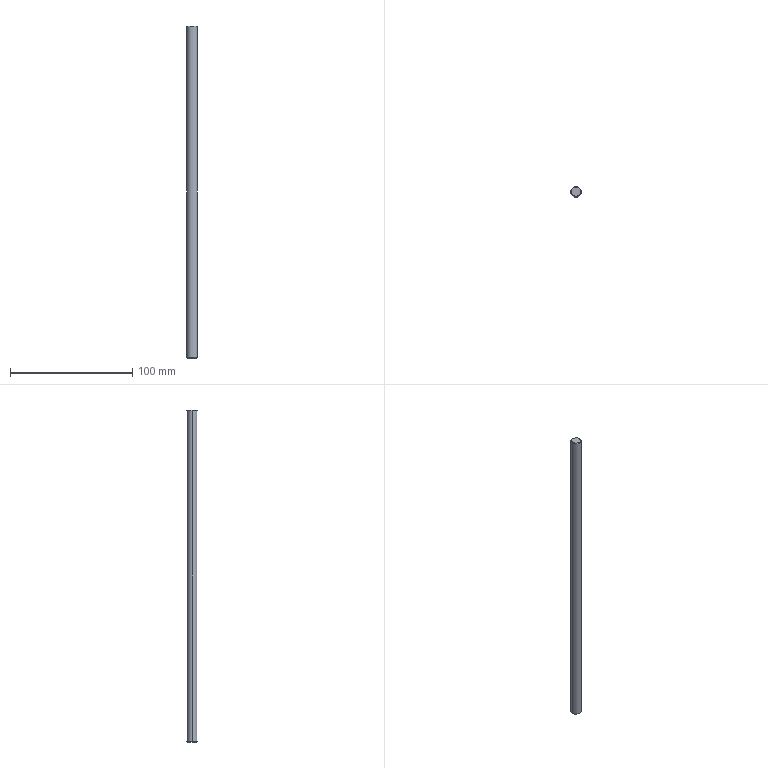Part | SolidWorks | features Chamfer 1, Extrusion 1 | 1 solid | 8 faces | box 8.5 x 8.5 x 271.5 mm | volume 15400 mm3 | cone 4 | cylinder 2 | plane 2 | commonest cylinder face diameters 8.5 x2
STEP:
#1=CARTESIAN_POINT('',(-3.75,0.,0.));
#2=VERTEX_POINT('',#1);
#3=CARTESIAN_POINT('',(3.75,0.,0.));
#4=VERTEX_POINT('',#3);
#5=CARTESIAN_POINT('',(0.,0.,0.));
#6=DIRECTION('',(0.,0.,-1.));
#7=DIRECTION('',(1.,0.,0.));
#8=AXIS2_PLACEMENT_3D('',#5,#6,#7);
#9=CIRCLE('',#8,3.75);
#10=EDGE_CURVE('',#2,#4,#9,.T.);
#11=ORIENTED_EDGE('',*,*,#10,.F.);
#12=CARTESIAN_POINT('',(-4.25,0.,0.5));
#13=VERTEX_POINT('',#12);
#14=CARTESIAN_POINT('',(-4.25,0.,0.5));
#15=DIRECTION('',(-0.7071,0.,0.7071));
#16=VECTOR('',#15,1000.);
#17=LINE('',#14,#16);
#18=EDGE_CURVE('',#2,#13,#17,.T.);
#19=ORIENTED_EDGE('',*,*,#18,.T.);
#20=CARTESIAN_POINT('',(4.25,0.,0.5));
#21=VERTEX_POINT('',#20);
#22=CARTESIAN_POINT('',(0.,0.,0.5));
#23=DIRECTION('',(0.,0.,1.));
#24=DIRECTION('',(1.,0.,0.));
#25=AXIS2_PLACEMENT_3D('',#22,#23,#24);
#26=CIRCLE('',#25,4.25);
#27=EDGE_CURVE('',#21,#13,#26,.T.);
#28=ORIENTED_EDGE('',*,*,#27,.F.);
#29=CARTESIAN_POINT('',(4.25,0.,0.5));
#30=DIRECTION('',(0.7071,0.,0.7071));
#31=VECTOR('',#30,1000.);
#32=LINE('',#29,#31);
#33=EDGE_CURVE('',#4,#21,#32,.T.);
#34=ORIENTED_EDGE('',*,*,#33,.F.);
#35=EDGE_LOOP('',(#11,#19,#28,#34));
#36=FACE_OUTER_BOUND('',#35,.T.);
#37=CARTESIAN_POINT('',(0.,0.,0.5));
#38=DIRECTION('',(0.,0.,1.));
#39=DIRECTION('',(1.,0.,0.));
#40=AXIS2_PLACEMENT_3D('',#37,#38,#39);
#41=CONICAL_SURFACE('',#40,4.25,0.7854);
#42=ADVANCED_FACE('',(#36),#41,.T.);
#43=CARTESIAN_POINT('',(3.75,0.,271.5));
#44=VERTEX_POINT('',#43);
#45=CARTESIAN_POINT('',(-3.75,0.,271.5));
#46=VERTEX_POINT('',#45);
#47=CARTESIAN_POINT('',(0.,0.,271.5));
#48=DIRECTION('',(0.,0.,1.));
#49=DIRECTION('',(1.,0.,0.));
#50=AXIS2_PLACEMENT_3D('',#47,#48,#49);
#51=CIRCLE('',#50,3.75);
#52=EDGE_CURVE('',#44,#46,#51,.T.);
#53=ORIENTED_EDGE('',*,*,#52,.F.);
#54=CARTESIAN_POINT('',(4.25,0.,271.));
#55=VERTEX_POINT('',#54);
#56=CARTESIAN_POINT('',(3.75,0.,271.5));
#57=DIRECTION('',(0.7071,0.,-0.7071));
#58=VECTOR('',#57,1000.);
#59=LINE('',#56,#58);
#60=EDGE_CURVE('',#44,#55,#59,.T.);
#61=ORIENTED_EDGE('',*,*,#60,.T.);
#62=CARTESIAN_POINT('',(-4.25,0.,271.));
#63=VERTEX_POINT('',#62);
#64=CARTESIAN_POINT('',(0.,0.,271.));
#65=DIRECTION('',(0.,0.,-1.));
#66=DIRECTION('',(1.,0.,0.));
#67=AXIS2_PLACEMENT_3D('',#64,#65,#66);
#68=CIRCLE('',#67,4.25);
#69=EDGE_CURVE('',#63,#55,#68,.T.);
#70=ORIENTED_EDGE('',*,*,#69,.F.);
#71=CARTESIAN_POINT('',(-3.75,0.,271.5));
#72=DIRECTION('',(-0.7071,0.,-0.7071));
#73=VECTOR('',#72,1000.);
#74=LINE('',#71,#73);
#75=EDGE_CURVE('',#46,#63,#74,.T.);
#76=ORIENTED_EDGE('',*,*,#75,.F.);
#77=EDGE_LOOP('',(#53,#61,#70,#76));
#78=FACE_OUTER_BOUND('',#77,.T.);
#79=CARTESIAN_POINT('',(0.,0.,271.5));
#80=DIRECTION('',(0.,0.,-1.));
#81=DIRECTION('',(-1.,0.,0.));
#82=AXIS2_PLACEMENT_3D('',#79,#80,#81);
#83=CONICAL_SURFACE('',#82,3.75,0.7854);
#84=ADVANCED_FACE('',(#78),#83,.T.);
#85=ORIENTED_EDGE('',*,*,#69,.T.);
#86=CARTESIAN_POINT('',(4.25,0.,271.5));
#87=DIRECTION('',(0.,0.,-1.));
#88=VECTOR('',#87,1000.);
#89=LINE('',#86,#88);
#90=EDGE_CURVE('',#55,#21,#89,.T.);
#91=ORIENTED_EDGE('',*,*,#90,.T.);
#92=ORIENTED_EDGE('',*,*,#27,.T.);
#93=CARTESIAN_POINT('',(-4.25,0.,271.5));
#94=DIRECTION('',(0.,0.,-1.));
#95=VECTOR('',#94,1000.);
#96=LINE('',#93,#95);
#97=EDGE_CURVE('',#63,#13,#96,.T.);
#98=ORIENTED_EDGE('',*,*,#97,.F.);
#99=EDGE_LOOP('',(#85,#91,#92,#98));
#100=FACE_OUTER_BOUND('',#99,.T.);
#101=CARTESIAN_POINT('',(0.,0.,271.5));
#102=DIRECTION('',(0.,0.,-1.));
#103=DIRECTION('',(-1.,0.,0.));
#104=AXIS2_PLACEMENT_3D('',#101,#102,#103);
#105=CYLINDRICAL_SURFACE('',#104,4.25);
#106=ADVANCED_FACE('',(#100),#105,.T.);
#107=ORIENTED_EDGE('',*,*,#90,.F.);
#108=CARTESIAN_POINT('',(0.,0.,271.));
#109=DIRECTION('',(0.,0.,-1.));
#110=DIRECTION('',(1.,0.,0.));
#111=AXIS2_PLACEMENT_3D('',#108,#109,#110);
#112=CIRCLE('',#111,4.25);
#113=EDGE_CURVE('',#55,#63,#112,.T.);
#114=ORIENTED_EDGE('',*,*,#113,.T.);
#115=ORIENTED_EDGE('',*,*,#97,.T.);
#116=CARTESIAN_POINT('',(0.,0.,0.5));
#117=DIRECTION('',(0.,0.,1.));
#118=DIRECTION('',(1.,0.,0.));
#119=AXIS2_PLACEMENT_3D('',#116,#117,#118);
#120=CIRCLE('',#119,4.25);
#121=EDGE_CURVE('',#13,#21,#120,.T.);
#122=ORIENTED_EDGE('',*,*,#121,.T.);
#123=EDGE_LOOP('',(#107,#114,#115,#122));
#124=FACE_OUTER_BOUND('',#123,.T.);
#125=CARTESIAN_POINT('',(0.,0.,271.5));
#126=DIRECTION('',(0.,0.,-1.));
#127=DIRECTION('',(-1.,0.,0.));
#128=AXIS2_PLACEMENT_3D('',#125,#126,#127);
#129=CYLINDRICAL_SURFACE('',#128,4.25);
#130=ADVANCED_FACE('',(#124),#129,.T.);
#131=CARTESIAN_POINT('',(0.,0.,271.5));
#132=DIRECTION('',(0.,0.,1.));
#133=DIRECTION('',(1.,0.,0.));
#134=AXIS2_PLACEMENT_3D('',#131,#132,#133);
#135=CIRCLE('',#134,3.75);
#136=EDGE_CURVE('',#46,#44,#135,.T.);
#137=ORIENTED_EDGE('',*,*,#136,.T.);
#138=ORIENTED_EDGE('',*,*,#52,.T.);
#139=EDGE_LOOP('',(#137,#138));
#140=FACE_OUTER_BOUND('',#139,.T.);
#141=CARTESIAN_POINT('',(0.,0.,271.5));
#142=DIRECTION('',(0.,0.,1.));
#143=DIRECTION('',(1.,0.,0.));
#144=AXIS2_PLACEMENT_3D('',#141,#142,#143);
#145=PLANE('',#144);
#146=ADVANCED_FACE('',(#140),#145,.T.);
#147=CARTESIAN_POINT('',(0.,0.,0.));
#148=DIRECTION('',(0.,0.,-1.));
#149=DIRECTION('',(1.,0.,0.));
#150=AXIS2_PLACEMENT_3D('',#147,#148,#149);
#151=CIRCLE('',#150,3.75);
#152=EDGE_CURVE('',#4,#2,#151,.T.);
#153=ORIENTED_EDGE('',*,*,#152,.T.);
#154=ORIENTED_EDGE('',*,*,#10,.T.);
#155=EDGE_LOOP('',(#153,#154));
#156=FACE_OUTER_BOUND('',#155,.T.);
#157=CARTESIAN_POINT('',(0.,0.,0.));
#158=DIRECTION('',(0.,0.,1.));
#159=DIRECTION('',(1.,0.,0.));
#160=AXIS2_PLACEMENT_3D('',#157,#158,#159);
#161=PLANE('',#160);
#162=ADVANCED_FACE('',(#156),#161,.F.);
#163=ORIENTED_EDGE('',*,*,#60,.F.);
#164=ORIENTED_EDGE('',*,*,#136,.F.);
#165=ORIENTED_EDGE('',*,*,#75,.T.);
#166=ORIENTED_EDGE('',*,*,#113,.F.);
#167=EDGE_LOOP('',(#163,#164,#165,#166));
#168=FACE_OUTER_BOUND('',#167,.T.);
#169=CARTESIAN_POINT('',(0.,0.,271.5));
#170=DIRECTION('',(0.,0.,-1.));
#171=DIRECTION('',(-1.,0.,0.));
#172=AXIS2_PLACEMENT_3D('',#169,#170,#171);
#173=CONICAL_SURFACE('',#172,3.75,0.7854);
#174=ADVANCED_FACE('',(#168),#173,.T.);
#175=ORIENTED_EDGE('',*,*,#18,.F.);
#176=ORIENTED_EDGE('',*,*,#152,.F.);
#177=ORIENTED_EDGE('',*,*,#33,.T.);
#178=ORIENTED_EDGE('',*,*,#121,.F.);
#179=EDGE_LOOP('',(#175,#176,#177,#178));
#180=FACE_OUTER_BOUND('',#179,.T.);
#181=CARTESIAN_POINT('',(0.,0.,0.5));
#182=DIRECTION('',(0.,0.,1.));
#183=DIRECTION('',(1.,0.,0.));
#184=AXIS2_PLACEMENT_3D('',#181,#182,#183);
#185=CONICAL_SURFACE('',#184,4.25,0.7854);
#186=ADVANCED_FACE('',(#180),#185,.T.);
#187=CLOSED_SHELL('',(#42,#84,#106,#130,#146,#162,#174,#186));
#188=MANIFOLD_SOLID_BREP('',#187);
#189=CARTESIAN_POINT('',(0.,0.,0.));
#190=DIRECTION('',(0.,0.,1.));
#191=DIRECTION('',(1.,0.,0.));
#192=AXIS2_PLACEMENT_3D('',#189,#190,#191);
#193=(LENGTH_UNIT()NAMED_UNIT(*)SI_UNIT(.MILLI.,.METRE.));
#194=UNCERTAINTY_MEASURE_WITH_UNIT(LENGTH_MEASURE(0.00001),#193,'','');
#195=(NAMED_UNIT(*)PLANE_ANGLE_UNIT()SI_UNIT($,.RADIAN.));
#196=(NAMED_UNIT(*)SI_UNIT($,.STERADIAN.)SOLID_ANGLE_UNIT());
#197=(GEOMETRIC_REPRESENTATION_CONTEXT(3)GLOBAL_UNCERTAINTY_ASSIGNED_CONTEXT((#194))GLOBAL_UNIT_ASSIGNED_CONTEXT((#193,#195,#196))REPRESENTATION_CONTEXT('',''));
#198=ADVANCED_BREP_SHAPE_REPRESENTATION('',(#188,#192),#197);